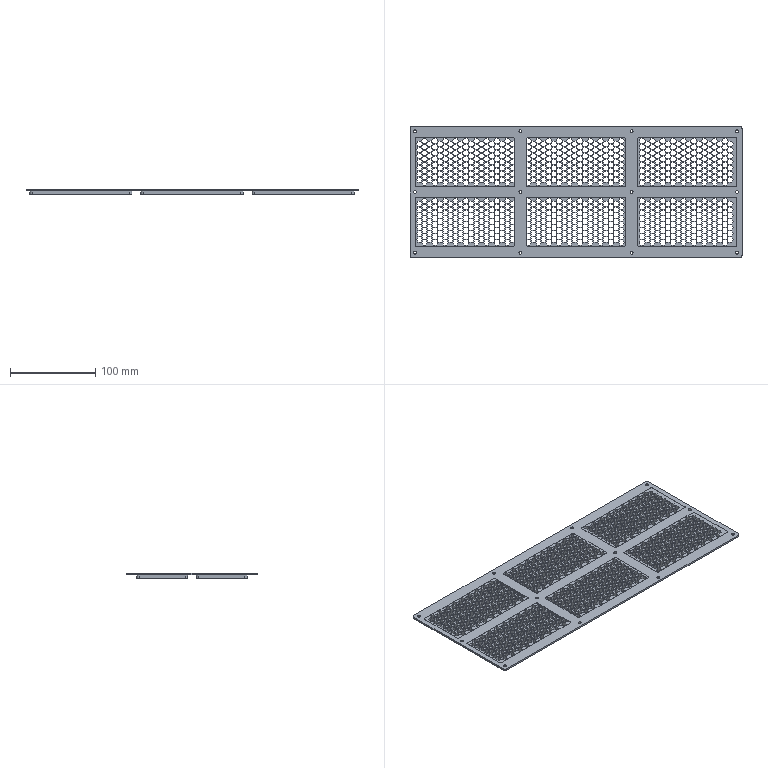NC program | NX | posted with a generic post
Lines 933 to 2108 of 7861:
(DRILLING_COPY_1 , TOOL : D4_CHAMFER)
N1822 T04 M6
N1824 G54
N1826 G17 G0 G90 X-183.338 Y56.437 S3000 M3
N1828 G43 Z30. H4
N1830 G94 G81 G98 Z-1.85 F200. R2.9
N1832 G80
N1834 G0 X-183.338 Y56.437 Z30.
(DRILLING_COPY_1_COPY_1 , TOOL : D4_CHAMFER)
N1836 X-171.218
N1838 G81 Z-1.85 F200. R2.9
N1840 G80
N1842 G0 X-171.218 Y56.437 Z30.
(DRILLING_COPY_1_COPY_2 , TOOL : D4_CHAMFER)
N1844 X-159.098
N1846 G81 Z-1.85 F200. R2.9
N1848 G80
N1850 G0 X-159.098 Y56.437 Z30.
(DRILLING_COPY_1_COPY_3 , TOOL : D4_CHAMFER)
N1852 X-146.978
N1854 G81 Z-1.85 F200. R2.9
N1856 G80
N1858 G0 X-146.978 Y56.437 Z30.
(DRILLING_COPY_1_COPY_4 , TOOL : D4_CHAMFER)
N1860 X-134.858
N1862 G81 Z-1.85 F200. R2.9
N1864 G80
N1866 G0 X-134.858 Y56.437 Z30.
(DRILLING_COPY_1_COPY_5 , TOOL : D4_CHAMFER)
N1868 X-122.738
N1870 G81 Z-1.85 F200. R2.9
N1872 G80
N1874 G0 X-122.738 Y56.437 Z30.
(DRILLING_COPY_1_COPY_6 , TOOL : D4_CHAMFER)
N1876 X-110.618
N1878 G81 Z-1.85 F200. R2.9
N1880 G80
N1882 G0 X-110.618 Y56.437 Z30.
(DRILLING_COPY_1_COPY_7 , TOOL : D4_CHAMFER)
N1884 X-98.498
N1886 G81 Z-1.85 F200. R2.9
N1888 G80
N1890 G0 X-98.498 Y56.437 Z30.
(DRILLING_COPY_1_COPY_8 , TOOL : D4_CHAMFER)
N1892 X-86.378
N1894 G81 Z-1.85 F200. R2.9
N1896 G80
N1898 G0 X-86.378 Y56.437 Z30.
(DRILLING_COPY_1_COPY_9 , TOOL : D4_CHAMFER)
N1900 X-183.338 Y49.437
N1902 G81 Z-1.85 F200. R2.9
N1904 G80
N1906 G0 X-183.338 Y49.437 Z30.
(DRILLING_COPY_1_COPY_1_COPY , TOOL : D4_CHAMFER)
N1908 X-171.218
N1910 G81 Z-1.85 F200. R2.9
N1912 G80
N1914 G0 X-171.218 Y49.437 Z30.
(DRILLING_COPY_1_COPY_2_COPY , TOOL : D4_CHAMFER)
N1916 X-159.098
N1918 G81 Z-1.85 F200. R2.9
N1920 G80
N1922 G0 X-159.098 Y49.437 Z30.
(DRILLING_COPY_1_COPY_3_COPY , TOOL : D4_CHAMFER)
N1924 X-146.978
N1926 G81 Z-1.85 F200. R2.9
N1928 G80
N1930 G0 X-146.978 Y49.437 Z30.
(DRILLING_COPY_1_COPY_4_COPY , TOOL : D4_CHAMFER)
N1932 X-134.858
N1934 G81 Z-1.85 F200. R2.9
N1936 G80
N1938 G0 X-134.858 Y49.437 Z30.
(DRILLING_COPY_1_COPY_5_COPY , TOOL : D4_CHAMFER)
N1940 X-122.738
N1942 G81 Z-1.85 F200. R2.9
N1944 G80
N1946 G0 X-122.738 Y49.437 Z30.
(DRILLING_COPY_1_COPY_6_COPY , TOOL : D4_CHAMFER)
N1948 X-110.618
N1950 G81 Z-1.85 F200. R2.9
N1952 G80
N1954 G0 X-110.618 Y49.437 Z30.
(DRILLING_COPY_1_COPY_7_COPY , TOOL : D4_CHAMFER)
N1956 X-98.498
N1958 G81 Z-1.85 F200. R2.9
N1960 G80
N1962 G0 X-98.498 Y49.437 Z30.
(DRILLING_COPY_1_COPY_8_COPY , TOOL : D4_CHAMFER)
N1964 X-86.378
N1966 G81 Z-1.85 F200. R2.9
N1968 G80
N1970 G0 X-86.378 Y49.437 Z30.
(DRILLING_COPY_1_COPY_10 , TOOL : D4_CHAMFER)
N1972 X-183.338 Y42.437
N1974 G81 Z-1.85 F200. R2.9
N1976 G80
N1978 G0 X-183.338 Y42.437 Z30.
(DRILLING_COPY_1_COPY_1_COPY_1 , TOOL : D4_CHAMFER)
N1980 X-171.218
N1982 G81 Z-1.85 F200. R2.9
N1984 G80
N1986 G0 X-171.218 Y42.437 Z30.
(DRILLING_COPY_1_COPY_2_COPY_1 , TOOL : D4_CHAMFER)
N1988 X-159.098
N1990 G81 Z-1.85 F200. R2.9
N1992 G80
N1994 G0 X-159.098 Y42.437 Z30.
(DRILLING_COPY_1_COPY_3_COPY_1 , TOOL : D4_CHAMFER)
N1996 X-146.978
N1998 G81 Z-1.85 F200. R2.9
N2000 G80
N2002 G0 X-146.978 Y42.437 Z30.
(DRILLING_COPY_1_COPY_4_COPY_1 , TOOL : D4_CHAMFER)
N2004 X-134.858
N2006 G81 Z-1.85 F200. R2.9
N2008 G80
N2010 G0 X-134.858 Y42.437 Z30.
(DRILLING_COPY_1_COPY_5_COPY_1 , TOOL : D4_CHAMFER)
N2012 X-122.738
N2014 G81 Z-1.85 F200. R2.9
N2016 G80
N2018 G0 X-122.738 Y42.437 Z30.
(DRILLING_COPY_1_COPY_6_COPY_1 , TOOL : D4_CHAMFER)
N2020 X-110.618
N2022 G81 Z-1.85 F200. R2.9
N2024 G80
N2026 G0 X-110.618 Y42.437 Z30.
(DRILLING_COPY_1_COPY_7_COPY_1 , TOOL : D4_CHAMFER)
N2028 X-98.498
N2030 G81 Z-1.85 F200. R2.9
N2032 G80
N2034 G0 X-98.498 Y42.437 Z30.
(DRILLING_COPY_1_COPY_8_COPY_1 , TOOL : D4_CHAMFER)
N2036 X-86.378
N2038 G81 Z-1.85 F200. R2.9
N2040 G80
N2042 G0 X-86.378 Y42.437 Z30.
(DRILLING_COPY_1_COPY_11 , TOOL : D4_CHAMFER)
N2044 X-183.338 Y35.437
N2046 G81 Z-1.85 F200. R2.9
N2048 G80
N2050 G0 X-183.338 Y35.437 Z30.
(DRILLING_COPY_1_COPY_1_COPY_2 , TOOL : D4_CHAMFER)
N2052 X-171.218
N2054 G81 Z-1.85 F200. R2.9
N2056 G80
N2058 G0 X-171.218 Y35.437 Z30.
(DRILLING_COPY_1_COPY_2_COPY_2 , TOOL : D4_CHAMFER)
N2060 X-159.098
N2062 G81 Z-1.85 F200. R2.9
N2064 G80
N2066 G0 X-159.098 Y35.437 Z30.
(DRILLING_COPY_1_COPY_3_COPY_2 , TOOL : D4_CHAMFER)
N2068 X-146.978
N2070 G81 Z-1.85 F200. R2.9
N2072 G80
N2074 G0 X-146.978 Y35.437 Z30.
(DRILLING_COPY_1_COPY_4_COPY_2 , TOOL : D4_CHAMFER)
N2076 X-134.858
N2078 G81 Z-1.85 F200. R2.9
N2080 G80
N2082 G0 X-134.858 Y35.437 Z30.
(DRILLING_COPY_1_COPY_5_COPY_2 , TOOL : D4_CHAMFER)
N2084 X-122.738
N2086 G81 Z-1.85 F200. R2.9
N2088 G80
N2090 G0 X-122.738 Y35.437 Z30.
(DRILLING_COPY_1_COPY_6_COPY_2 , TOOL : D4_CHAMFER)
N2092 X-110.618
N2094 G81 Z-1.85 F200. R2.9
N2096 G80
N2098 G0 X-110.618 Y35.437 Z30.
(DRILLING_COPY_1_COPY_7_COPY_2 , TOOL : D4_CHAMFER)
N2100 X-98.498
N2102 G81 Z-1.85 F200. R2.9
N2104 G80
N2106 G0 X-98.498 Y35.437 Z30.
(DRILLING_COPY_1_COPY_8_COPY_2 , TOOL : D4_CHAMFER)
N2108 X-86.378
N2110 G81 Z-1.85 F200. R2.9
N2112 G80
N2114 G0 X-86.378 Y35.437 Z30.
(DRILLING_COPY_1_COPY_12 , TOOL : D4_CHAMFER)
N2116 X-183.338 Y28.437
N2118 G81 Z-1.85 F200. R2.9
N2120 G80
N2122 G0 X-183.338 Y28.437 Z30.
(DRILLING_COPY_1_COPY_1_COPY_3 , TOOL : D4_CHAMFER)
N2124 X-171.218
N2126 G81 Z-1.85 F200. R2.9
N2128 G80
N2130 G0 X-171.218 Y28.437 Z30.
(DRILLING_COPY_1_COPY_2_COPY_3 , TOOL : D4_CHAMFER)
N2132 X-159.098
N2134 G81 Z-1.85 F200. R2.9
N2136 G80
N2138 G0 X-159.098 Y28.437 Z30.
(DRILLING_COPY_1_COPY_3_COPY_3 , TOOL : D4_CHAMFER)
N2140 X-146.978
N2142 G81 Z-1.85 F200. R2.9
N2144 G80
N2146 G0 X-146.978 Y28.437 Z30.
(DRILLING_COPY_1_COPY_4_COPY_3 , TOOL : D4_CHAMFER)
N2148 X-134.858
N2150 G81 Z-1.85 F200. R2.9
N2152 G80
N2154 G0 X-134.858 Y28.437 Z30.
(DRILLING_COPY_1_COPY_5_COPY_3 , TOOL : D4_CHAMFER)
N2156 X-122.738
N2158 G81 Z-1.85 F200. R2.9
N2160 G80
N2162 G0 X-122.738 Y28.437 Z30.
(DRILLING_COPY_1_COPY_6_COPY_3 , TOOL : D4_CHAMFER)
N2164 X-110.618
N2166 G81 Z-1.85 F200. R2.9
N2168 G80
N2170 G0 X-110.618 Y28.437 Z30.
(DRILLING_COPY_1_COPY_7_COPY_3 , TOOL : D4_CHAMFER)
N2172 X-98.498
N2174 G81 Z-1.85 F200. R2.9
N2176 G80
N2178 G0 X-98.498 Y28.437 Z30.
(DRILLING_COPY_1_COPY_8_COPY_3 , TOOL : D4_CHAMFER)
N2180 X-86.378
N2182 G81 Z-1.85 F200. R2.9
N2184 G80
N2186 G0 X-86.378 Y28.437 Z30.
(DRILLING_COPY_1_COPY_13 , TOOL : D4_CHAMFER)
N2188 X-183.338 Y21.437
N2190 G81 Z-1.85 F200. R2.9
N2192 G80
N2194 G0 X-183.338 Y21.437 Z30.
(DRILLING_COPY_1_COPY_1_COPY_4 , TOOL : D4_CHAMFER)
N2196 X-171.218
N2198 G81 Z-1.85 F200. R2.9
N2200 G80
N2202 G0 X-171.218 Y21.437 Z30.
(DRILLING_COPY_1_COPY_2_COPY_4 , TOOL : D4_CHAMFER)
N2204 X-159.098
N2206 G81 Z-1.85 F200. R2.9
N2208 G80
N2210 G0 X-159.098 Y21.437 Z30.
(DRILLING_COPY_1_COPY_3_COPY_4 , TOOL : D4_CHAMFER)
N2212 X-146.978
N2214 G81 Z-1.85 F200. R2.9
N2216 G80
N2218 G0 X-146.978 Y21.437 Z30.
(DRILLING_COPY_1_COPY_4_COPY_4 , TOOL : D4_CHAMFER)
N2220 X-134.858
N2222 G81 Z-1.85 F200. R2.9
N2224 G80
N2226 G0 X-134.858 Y21.437 Z30.
(DRILLING_COPY_1_COPY_5_COPY_4 , TOOL : D4_CHAMFER)
N2228 X-122.738
N2230 G81 Z-1.85 F200. R2.9
N2232 G80
N2234 G0 X-122.738 Y21.437 Z30.
(DRILLING_COPY_1_COPY_6_COPY_4 , TOOL : D4_CHAMFER)
N2236 X-110.618
N2238 G81 Z-1.85 F200. R2.9
N2240 G80
N2242 G0 X-110.618 Y21.437 Z30.
(DRILLING_COPY_1_COPY_7_COPY_4 , TOOL : D4_CHAMFER)
N2244 X-98.498
N2246 G81 Z-1.85 F200. R2.9
N2248 G80
N2250 G0 X-98.498 Y21.437 Z30.
(DRILLING_COPY_1_COPY_8_COPY_4 , TOOL : D4_CHAMFER)
N2252 X-86.378
N2254 G81 Z-1.85 F200. R2.9
N2256 G80
N2258 G0 X-86.378 Y21.437 Z30.
(DRILLING_COPY_1_COPY_14 , TOOL : D4_CHAMFER)
N2260 X-183.338 Y14.437
N2262 G81 Z-1.85 F200. R2.9
N2264 G80
N2266 G0 X-183.338 Y14.437 Z30.
(DRILLING_COPY_1_COPY_1_COPY_5 , TOOL : D4_CHAMFER)
N2268 X-171.218
N2270 G81 Z-1.85 F200. R2.9
N2272 G80
N2274 G0 X-171.218 Y14.437 Z30.
(DRILLING_COPY_1_COPY_2_COPY_5 , TOOL : D4_CHAMFER)
N2276 X-159.098
N2278 G81 Z-1.85 F200. R2.9
N2280 G80
N2282 G0 X-159.098 Y14.437 Z30.
(DRILLING_COPY_1_COPY_3_COPY_5 , TOOL : D4_CHAMFER)
N2284 X-146.978
N2286 G81 Z-1.85 F200. R2.9
N2288 G80
N2290 G0 X-146.978 Y14.437 Z30.
(DRILLING_COPY_1_COPY_4_COPY_5 , TOOL : D4_CHAMFER)
N2292 X-134.858
N2294 G81 Z-1.85 F200. R2.9
N2296 G80
N2298 G0 X-134.858 Y14.437 Z30.
(DRILLING_COPY_1_COPY_5_COPY_5 , TOOL : D4_CHAMFER)
N2300 X-122.738
N2302 G81 Z-1.85 F200. R2.9
N2304 G80
N2306 G0 X-122.738 Y14.437 Z30.
(DRILLING_COPY_1_COPY_6_COPY_5 , TOOL : D4_CHAMFER)
N2308 X-110.618
N2310 G81 Z-1.85 F200. R2.9
N2312 G80
N2314 G0 X-110.618 Y14.437 Z30.
(DRILLING_COPY_1_COPY_7_COPY_5 , TOOL : D4_CHAMFER)
N2316 X-98.498
N2318 G81 Z-1.85 F200. R2.9
N2320 G80
N2322 G0 X-98.498 Y14.437 Z30.
(DRILLING_COPY_1_COPY_8_COPY_5 , TOOL : D4_CHAMFER)
N2324 X-86.378
N2326 G81 Z-1.85 F200. R2.9
N2328 G80
N2330 G0 X-86.378 Y14.437 Z30.
(DRILLING_COPY_1_COPY , TOOL : D4_CHAMFER)
N2332 X-177.276 Y59.937
N2334 G81 Z-1.85 F200. R2.9
N2336 G80
N2338 G0 X-177.276 Y59.937 Z30.
(DRILLING_COPY_1_COPY_COPY , TOOL : D4_CHAMFER)
N2340 X-165.156
N2342 G81 Z-1.85 F200. R2.9
N2344 G80
N2346 G0 X-165.156 Y59.937 Z30.
(DRILLING_COPY_1_COPY_COPY_1 , TOOL : D4_CHAMFER)
N2348 X-153.036
N2350 G81 Z-1.85 F200. R2.9
N2352 G80
N2354 G0 X-153.036 Y59.937 Z30.
(DRILLING_COPY_1_COPY_COPY_2 , TOOL : D4_CHAMFER)
N2356 X-140.916
N2358 G81 Z-1.85 F200. R2.9
N2360 G80
N2362 G0 X-140.916 Y59.937 Z30.
(DRILLING_COPY_1_COPY_COPY_3 , TOOL : D4_CHAMFER)
N2364 X-128.796
N2366 G81 Z-1.85 F200. R2.9
N2368 G80
N2370 G0 X-128.796 Y59.937 Z30.
(DRILLING_COPY_1_COPY_COPY_4 , TOOL : D4_CHAMFER)
N2372 X-116.676
N2374 G81 Z-1.85 F200. R2.9
N2376 G80
N2378 G0 X-116.676 Y59.937 Z30.
(DRILLING_COPY_1_COPY_COPY_5 , TOOL : D4_CHAMFER)
N2380 X-104.556
N2382 G81 Z-1.85 F200. R2.9
N2384 G80
N2386 G0 X-104.556 Y59.937 Z30.
(DRILLING_COPY_1_COPY_COPY_6 , TOOL : D4_CHAMFER)
N2388 X-92.436
N2390 G81 Z-1.85 F200. R2.9
N2392 G80
N2394 G0 X-92.436 Y59.937 Z30.
(DRILLING_COPY_1_COPY_COPY_7 , TOOL : D4_CHAMFER)
N2396 X-80.316
N2398 G81 Z-1.85 F200. R2.9
N2400 G80
N2402 G0 X-80.316 Y59.937 Z30.
(DRILLING_COPY_1_COPY_COPY_8 , TOOL : D4_CHAMFER)
N2404 X-177.276 Y52.937
N2406 G81 Z-1.85 F200. R2.9
N2408 G80
N2410 G0 X-177.276 Y52.937 Z30.
(DRILLING_COPY_1_COPY_COPY_COPY , TOOL : D4_CHAMFER)
N2412 X-165.156
N2414 G81 Z-1.85 F200. R2.9
N2416 G80
N2418 G0 X-165.156 Y52.937 Z30.
(DRILLING_COPY_1_COPY_COPY_1_COPY , TOOL : D4_CHAMFER)
N2420 X-153.036
N2422 G81 Z-1.85 F200. R2.9
N2424 G80
N2426 G0 X-153.036 Y52.937 Z30.
(DRILLING_COPY_1_COPY_COPY_2_COPY , TOOL : D4_CHAMFER)
N2428 X-140.916
N2430 G81 Z-1.85 F200. R2.9
N2432 G80
N2434 G0 X-140.916 Y52.937 Z30.
(DRILLING_COPY_1_COPY_COPY_3_COPY , TOOL : D4_CHAMFER)
N2436 X-128.796
N2438 G81 Z-1.85 F200. R2.9
N2440 G80
N2442 G0 X-128.796 Y52.937 Z30.
(DRILLING_COPY_1_COPY_COPY_4_COPY , TOOL : D4_CHAMFER)
N2444 X-116.676
N2446 G81 Z-1.85 F200. R2.9
N2448 G80
N2450 G0 X-116.676 Y52.937 Z30.
(DRILLING_COPY_1_COPY_COPY_5_COPY , TOOL : D4_CHAMFER)
N2452 X-104.556
N2454 G81 Z-1.85 F200. R2.9
N2456 G80
N2458 G0 X-104.556 Y52.937 Z30.
(DRILLING_COPY_1_COPY_COPY_6_COPY , TOOL : D4_CHAMFER)
N2460 X-92.436
N2462 G81 Z-1.85 F200. R2.9
N2464 G80
N2466 G0 X-92.436 Y52.937 Z30.
(DRILLING_COPY_1_COPY_COPY_7_COPY , TOOL : D4_CHAMFER)
N2468 X-80.316
N2470 G81 Z-1.85 F200. R2.9
N2472 G80
N2474 G0 X-80.316 Y52.937 Z30.
(DRILLING_COPY_1_COPY_COPY_9 , TOOL : D4_CHAMFER)
N2476 X-177.276 Y45.937
N2478 G81 Z-1.85 F200. R2.9
N2480 G80
N2482 G0 X-177.276 Y45.937 Z30.
(DRILLING_COPY_1_COPY_COPY_COPY_1 , TOOL : D4_CHAMFER)
N2484 X-165.156
N2486 G81 Z-1.85 F200. R2.9
N2488 G80
N2490 G0 X-165.156 Y45.937 Z30.
(DRILLING_COPY_1_COPY_COPY_1_COPY_1 , TOOL : D4_CHAMFER)
N2492 X-153.036
N2494 G81 Z-1.85 F200. R2.9
N2496 G80
N2498 G0 X-153.036 Y45.937 Z30.
(DRILLING_COPY_1_COPY_COPY_2_COPY_1 , TOOL : D4_CHAMFER)
N2500 X-140.916
N2502 G81 Z-1.85 F200. R2.9
N2504 G80
N2506 G0 X-140.916 Y45.937 Z30.
(DRILLING_COPY_1_COPY_COPY_3_COPY_1 , TOOL : D4_CHAMFER)
N2508 X-128.796
N2510 G81 Z-1.85 F200. R2.9
N2512 G80
N2514 G0 X-128.796 Y45.937 Z30.
(DRILLING_COPY_1_COPY_COPY_4_COPY_1 , TOOL : D4_CHAMFER)
N2516 X-116.676
N2518 G81 Z-1.85 F200. R2.9
N2520 G80
N2522 G0 X-116.676 Y45.937 Z30.
(DRILLING_COPY_1_COPY_COPY_5_COPY_1 , TOOL : D4_CHAMFER)
N2524 X-104.556
N2526 G81 Z-1.85 F200. R2.9
N2528 G80
N2530 G0 X-104.556 Y45.937 Z30.
(DRILLING_COPY_1_COPY_COPY_6_COPY_1 , TOOL : D4_CHAMFER)
N2532 X-92.436
N2534 G81 Z-1.85 F200. R2.9
N2536 G80
N2538 G0 X-92.436 Y45.937 Z30.
(DRILLING_COPY_1_COPY_COPY_7_COPY_1 , TOOL : D4_CHAMFER)
N2540 X-80.316
N2542 G81 Z-1.85 F200. R2.9
N2544 G80
N2546 G0 X-80.316 Y45.937 Z30.
(DRILLING_COPY_1_COPY_COPY_10 , TOOL : D4_CHAMFER)
N2548 X-177.276 Y38.937
N2550 G81 Z-1.85 F200. R2.9
N2552 G80
N2554 G0 X-177.276 Y38.937 Z30.
(DRILLING_COPY_1_COPY_COPY_COPY_2 , TOOL : D4_CHAMFER)
N2556 X-165.156
N2558 G81 Z-1.85 F200. R2.9
N2560 G80
N2562 G0 X-165.156 Y38.937 Z30.
(DRILLING_COPY_1_COPY_COPY_1_COPY_2 , TOOL : D4_CHAMFER)
N2564 X-153.036
N2566 G81 Z-1.85 F200. R2.9
N2568 G80
N2570 G0 X-153.036 Y38.937 Z30.
(DRILLING_COPY_1_COPY_COPY_2_COPY_2 , TOOL : D4_CHAMFER)
N2572 X-140.916
N2574 G81 Z-1.85 F200. R2.9
N2576 G80
N2578 G0 X-140.916 Y38.937 Z30.
(DRILLING_COPY_1_COPY_COPY_3_COPY_2 , TOOL : D4_CHAMFER)
N2580 X-128.796
N2582 G81 Z-1.85 F200. R2.9
N2584 G80
N2586 G0 X-128.796 Y38.937 Z30.
(DRILLING_COPY_1_COPY_COPY_4_COPY_2 , TOOL : D4_CHAMFER)
N2588 X-116.676
N2590 G81 Z-1.85 F200. R2.9
N2592 G80
N2594 G0 X-116.676 Y38.937 Z30.
(DRILLING_COPY_1_COPY_COPY_5_COPY_2 , TOOL : D4_CHAMFER)
N2596 X-104.556
N2598 G81 Z-1.85 F200. R2.9
N2600 G80
N2602 G0 X-104.556 Y38.937 Z30.
(DRILLING_COPY_1_COPY_COPY_6_COPY_2 , TOOL : D4_CHAMFER)
N2604 X-92.436
N2606 G81 Z-1.85 F200. R2.9
N2608 G80
N2610 G0 X-92.436 Y38.937 Z30.
(DRILLING_COPY_1_COPY_COPY_7_COPY_2 , TOOL : D4_CHAMFER)
N2612 X-80.316
N2614 G81 Z-1.85 F200. R2.9
N2616 G80
N2618 G0 X-80.316 Y38.937 Z30.
(DRILLING_COPY_1_COPY_COPY_11 , TOOL : D4_CHAMFER)
N2620 X-177.276 Y31.937
N2622 G81 Z-1.85 F200. R2.9
N2624 G80
N2626 G0 X-177.276 Y31.937 Z30.
(DRILLING_COPY_1_COPY_COPY_COPY_3 , TOOL : D4_CHAMFER)
N2628 X-165.156
N2630 G81 Z-1.85 F200. R2.9
N2632 G80
N2634 G0 X-165.156 Y31.937 Z30.
(DRILLING_COPY_1_COPY_COPY_1_COPY_3 , TOOL : D4_CHAMFER)
N2636 X-153.036
N2638 G81 Z-1.85 F200. R2.9
N2640 G80
N2642 G0 X-153.036 Y31.937 Z30.
(DRILLING_COPY_1_COPY_COPY_2_COPY_3 , TOOL : D4_CHAMFER)
N2644 X-140.916
N2646 G81 Z-1.85 F200. R2.9
N2648 G80
N2650 G0 X-140.916 Y31.937 Z30.
(DRILLING_COPY_1_COPY_COPY_3_COPY_3 , TOOL : D4_CHAMFER)
N2652 X-128.796
N2654 G81 Z-1.85 F200. R2.9
N2656 G80
N2658 G0 X-128.796 Y31.937 Z30.
(DRILLING_COPY_1_COPY_COPY_4_COPY_3 , TOOL : D4_CHAMFER)
N2660 X-116.676
N2662 G81 Z-1.85 F200. R2.9
N2664 G80
N2666 G0 X-116.676 Y31.937 Z30.
(DRILLING_COPY_1_COPY_COPY_5_COPY_3 , TOOL : D4_CHAMFER)
N2668 X-104.556
N2670 G81 Z-1.85 F200. R2.9
N2672 G80
N2674 G0 X-104.556 Y31.937 Z30.
(DRILLING_COPY_1_COPY_COPY_6_COPY_3 , TOOL : D4_CHAMFER)
N2676 X-92.436
N2678 G81 Z-1.85 F200. R2.9
N2680 G80
N2682 G0 X-92.436 Y31.937 Z30.
(DRILLING_COPY_1_COPY_COPY_7_COPY_3 , TOOL : D4_CHAMFER)
N2684 X-80.316
N2686 G81 Z-1.85 F200. R2.9
N2688 G80
N2690 G0 X-80.316 Y31.937 Z30.
(DRILLING_COPY_1_COPY_COPY_12 , TOOL : D4_CHAMFER)
N2692 X-177.276 Y24.937
N2694 G81 Z-1.85 F200. R2.9
N2696 G80
N2698 G0 X-177.276 Y24.937 Z30.
(DRILLING_COPY_1_COPY_COPY_COPY_4 , TOOL : D4_CHAMFER)
N2700 X-165.156
N2702 G81 Z-1.85 F200. R2.9
N2704 G80
N2706 G0 X-165.156 Y24.937 Z30.
(DRILLING_COPY_1_COPY_COPY_1_COPY_4 , TOOL : D4_CHAMFER)
N2708 X-153.036
N2710 G81 Z-1.85 F200. R2.9
N2712 G80
N2714 G0 X-153.036 Y24.937 Z30.
(DRILLING_COPY_1_COPY_COPY_2_COPY_4 , TOOL : D4_CHAMFER)
N2716 X-140.916
N2718 G81 Z-1.85 F200. R2.9
N2720 G80
N2722 G0 X-140.916 Y24.937 Z30.
(DRILLING_COPY_1_COPY_COPY_3_COPY_4 , TOOL : D4_CHAMFER)
N2724 X-128.796
N2726 G81 Z-1.85 F200. R2.9
N2728 G80
N2730 G0 X-128.796 Y24.937 Z30.
(DRILLING_COPY_1_COPY_COPY_4_COPY_4 , TOOL : D4_CHAMFER)
N2732 X-116.676
N2734 G81 Z-1.85 F200. R2.9
N2736 G80
N2738 G0 X-116.676 Y24.937 Z30.
(DRILLING_COPY_1_COPY_COPY_5_COPY_4 , TOOL : D4_CHAMFER)
N2740 X-104.556
N2742 G81 Z-1.85 F200. R2.9
N2744 G80
N2746 G0 X-104.556 Y24.937 Z30.
(DRILLING_COPY_1_COPY_COPY_6_COPY_4 , TOOL : D4_CHAMFER)
N2748 X-92.436
N2750 G81 Z-1.85 F200. R2.9
N2752 G80
N2754 G0 X-92.436 Y24.937 Z30.
(DRILLING_COPY_1_COPY_COPY_7_COPY_4 , TOOL : D4_CHAMFER)
N2756 X-80.316
N2758 G81 Z-1.85 F200. R2.9
N2760 G80
N2762 G0 X-80.316 Y24.937 Z30.
(DRILLING_COPY_1_COPY_COPY_13 , TOOL : D4_CHAMFER)
N2764 X-177.276 Y17.937
N2766 G81 Z-1.85 F200. R2.9
N2768 G80
N2770 G0 X-177.276 Y17.937 Z30.
(DRILLING_COPY_1_COPY_COPY_COPY_5 , TOOL : D4_CHAMFER)
N2772 X-165.156
N2774 G81 Z-1.85 F200. R2.9
N2776 G80
N2778 G0 X-165.156 Y17.937 Z30.
(DRILLING_COPY_1_COPY_COPY_1_COPY_5 , TOOL : D4_CHAMFER)
N2780 X-153.036
N2782 G81 Z-1.85 F200. R2.9
N2784 G80
N2786 G0 X-153.036 Y17.937 Z30.
(DRILLING_COPY_1_COPY_COPY_2_COPY_5 , TOOL : D4_CHAMFER)
N2788 X-140.916
N2790 G81 Z-1.85 F200. R2.9
N2792 G80
N2794 G0 X-140.916 Y17.937 Z30.
(DRILLING_COPY_1_COPY_COPY_3_COPY_5 , TOOL : D4_CHAMFER)
N2796 X-128.796
N2798 G81 Z-1.85 F200. R2.9
N2800 G80
N2802 G0 X-128.796 Y17.937 Z30.
(DRILLING_COPY_1_COPY_COPY_4_COPY_5 , TOOL : D4_CHAMFER)
N2804 X-116.676
N2806 G81 Z-1.85 F200. R2.9
N2808 G80
N2810 G0 X-116.676 Y17.937 Z30.
(DRILLING_COPY_1_COPY_COPY_5_COPY_5 , TOOL : D4_CHAMFER)
N2812 X-104.556
N2814 G81 Z-1.85 F200. R2.9
N2816 G80
N2818 G0 X-104.556 Y17.937 Z30.
(DRILLING_COPY_1_COPY_COPY_6_COPY_5 , TOOL : D4_CHAMFER)
N2820 X-92.436
N2822 G81 Z-1.85 F200. R2.9
N2824 G80
N2826 G0 X-92.436 Y17.937 Z30.
(DRILLING_COPY_1_COPY_COPY_7_COPY_5 , TOOL : D4_CHAMFER)
N2828 X-80.316
N2830 G81 Z-1.85 F200. R2.9
N2832 G80
N2834 G0 X-80.316 Y17.937 Z30.
(DRILLING_COPY_1_COPY_COPY_14 , TOOL : D4_CHAMFER)
N2836 X-177.276 Y10.937
N2838 G81 Z-1.85 F200. R2.9
N2840 G80
N2842 G0 X-177.276 Y10.937 Z30.
(DRILLING_COPY_1_COPY_COPY_COPY_6 , TOOL : D4_CHAMFER)
N2844 X-165.156
N2846 G81 Z-1.85 F200. R2.9
N2848 G80
N2850 G0 X-165.156 Y10.937 Z30.
(DRILLING_COPY_1_COPY_COPY_1_COPY_6 , TOOL : D4_CHAMFER)
N2852 X-153.036
N2854 G81 Z-1.85 F200. R2.9
N2856 G80
N2858 G0 X-153.036 Y10.937 Z30.
(DRILLING_COPY_1_COPY_COPY_2_COPY_6 , TOOL : D4_CHAMFER)
N2860 X-140.916
N2862 G81 Z-1.85 F200. R2.9
N2864 G80
N2866 G0 X-140.916 Y10.937 Z30.
(DRILLING_COPY_1_COPY_COPY_3_COPY_6 , TOOL : D4_CHAMFER)
N2868 X-128.796
N2870 G81 Z-1.85 F200. R2.9
N2872 G80
N2874 G0 X-128.796 Y10.937 Z30.
(DRILLING_COPY_1_COPY_COPY_4_COPY_6 , TOOL : D4_CHAMFER)
N2876 X-116.676
N2878 G81 Z-1.85 F200. R2.9
N2880 G80
N2882 G0 X-116.676 Y10.937 Z30.
(DRILLING_COPY_1_COPY_COPY_5_COPY_6 , TOOL : D4_CHAMFER)
N2884 X-104.556
N2886 G81 Z-1.85 F200. R2.9
N2888 G80
N2890 G0 X-104.556 Y10.937 Z30.
(DRILLING_COPY_1_COPY_COPY_6_COPY_6 , TOOL : D4_CHAMFER)
N2892 X-92.436
N2894 G81 Z-1.85 F200. R2.9
N2896 G80
N2898 G0 X-92.436 Y10.937 Z30.
(DRILLING_COPY_1_COPY_COPY_7_COPY_6 , TOOL : D4_CHAMFER)
N2900 X-80.316
N2902 G81 Z-1.85 F200. R2.9
N2904 G80
N2906 G0 X-80.316 Y10.937 Z30.
(DRILLING_COPY_1_COPY_15 , TOOL : D4_CHAMFER)
N2908 X-74.218 Y56.437
N2910 G81 Z-1.85 F200. R2.9
N2912 G80
N2914 G0 X-74.218 Y56.437 Z30.
(DRILLING_COPY_1_COPY_15_COPY , TOOL : D4_CHAMFER)
N2916 Y49.437
N2918 G81 Z-1.85 F200. R2.9
N2920 G80
N2922 G0 X-74.218 Y49.437 Z30.
(DRILLING_COPY_1_COPY_15_COPY_1 , TOOL : D4_CHAMFER)
N2924 Y42.437
N2926 G81 Z-1.85 F200. R2.9
N2928 G80
N2930 G0 X-74.218 Y42.437 Z30.
(DRILLING_COPY_1_COPY_15_COPY_2 , TOOL : D4_CHAMFER)
N2932 Y35.437
N2934 G81 Z-1.85 F200. R2.9
N2936 G80
N2938 G0 X-74.218 Y35.437 Z30.
(DRILLING_COPY_1_COPY_15_COPY_3 , TOOL : D4_CHAMFER)
N2940 Y28.437
N2942 G81 Z-1.85 F200. R2.9
N2944 G80
N2946 G0 X-74.218 Y28.437 Z30.
(DRILLING_COPY_1_COPY_15_COPY_4 , TOOL : D4_CHAMFER)
N2948 Y21.437
N2950 G81 Z-1.85 F200. R2.9
N2952 G80
N2954 G0 X-74.218 Y21.437 Z30.
(DRILLING_COPY_1_COPY_15_COPY_5 , TOOL : D4_CHAMFER)
N2956 Y14.437
N2958 G81 Z-1.85 F200. R2.9
N2960 G80
N2962 G0 X-74.218 Y14.437 Z30.
(DRILLING_COPY_1_COPY_15_COPY_6 , TOOL : D4_CHAMFER)
N2964 X-183.338 Y-55.563
N2966 G81 Z-1.85 F200. R2.9
N2968 G80
N2970 G0 X-183.338 Y-55.563 Z30.
(DRILLING_COPY_1_COPY_15_COPY_6_COPY , TOOL : D4_CHAMFER)
N2972 Y-48.563
N2974 G81 Z-1.85 F200. R2.9
N2976 G80
N2978 G0 X-183.338 Y-48.563 Z30.
(DRILLING_COPY_1_COPY_15_COPY_6_COPY_1 , TOOL : D4_CHAMFER)
N2980 Y-41.563
N2982 G81 Z-1.85 F200. R2.9
N2984 G80
N2986 G0 X-183.338 Y-41.563 Z30.
(DRILLING_COPY_1_COPY_15_COPY_6_COPY_2 , TOOL : D4_CHAMFER)
N2988 Y-34.563
N2990 G81 Z-1.85 F200. R2.9
N2992 G80
N2994 G0 X-183.338 Y-34.563 Z30.
(DRILLING_COPY_1_COPY_15_COPY_6_COPY_3 , TOOL : D4_CHAMFER)
N2996 Y-27.563
N2998 G81 Z-1.85 F200. R2.9
N3000 G80
N3002 G0 X-183.338 Y-27.563 Z30.
(DRILLING_COPY_1_COPY_15_COPY_6_COPY_4 , TOOL : D4_CHAMFER)
N3004 Y-20.563
N3006 G81 Z-1.85 F200. R2.9
N3008 G80
N3010 G0 X-183.338 Y-20.563 Z30.
(DRILLING_COPY_1_COPY_15_COPY_6_COPY_5 , TOOL : D4_CHAMFER)
N3012 Y-13.563
N3014 G81 Z-1.85 F200. R2.9
N3016 G80
N3018 G0 X-183.338 Y-13.563 Z30.
(DRILLING_COPY_1_COPY_15_COPY_6_COPY_6 , TOOL : D4_CHAMFER)
N3020 X-171.218 Y-55.563
N3022 G81 Z-1.85 F200. R2.9
N3024 G80
N3026 G0 X-171.218 Y-55.563 Z30.
(DRILLING_COPY_1_COPY_15_COPY_6_COPY_COPY , TOOL : D4_CHAMFER)
N3028 Y-48.563
N3030 G81 Z-1.85 F200. R2.9
N3032 G80
N3034 G0 X-171.218 Y-48.563 Z30.
(DRILLING_COPY_1_COPY_15_COPY_6_COPY_1_COPY , TOOL : D4_CHAMFER)
N3036 Y-41.563
N3038 G81 Z-1.85 F200. R2.9
N3040 G80
N3042 G0 X-171.218 Y-41.563 Z30.
(DRILLING_COPY_1_COPY_15_COPY_6_COPY_2_COPY , TOOL : D4_CHAMFER)
N3044 Y-34.563
N3046 G81 Z-1.85 F200. R2.9
N3048 G80
N3050 G0 X-171.218 Y-34.563 Z30.
(DRILLING_COPY_1_COPY_15_COPY_6_COPY_3_COPY , TOOL : D4_CHAMFER)
N3052 Y-27.563
N3054 G81 Z-1.85 F200. R2.9
N3056 G80
N3058 G0 X-171.218 Y-27.563 Z30.
(DRILLING_COPY_1_COPY_15_COPY_6_COPY_4_COPY , TOOL : D4_CHAMFER)
N3060 Y-20.563
N3062 G81 Z-1.85 F200. R2.9
N3064 G80
N3066 G0 X-171.218 Y-20.563 Z30.
(DRILLING_COPY_1_COPY_15_COPY_6_COPY_5_COPY , TOOL : D4_CHAMFER)
N3068 Y-13.563
N3070 G81 Z-1.85 F200. R2.9
N3072 G80
N3074 G0 X-171.218 Y-13.563 Z30.
(DRILLING_COPY_1_COPY_15_COPY_6_COPY_7 , TOOL : D4_CHAMFER)
N3076 X-159.098 Y-55.563
N3078 G81 Z-1.85 F200. R2.9
N3080 G80
N3082 G0 X-159.098 Y-55.563 Z30.
(DRILLING_COPY_1_COPY_15_COPY_6_COPY_COPY_1 , TOOL : D4_CHAMFER)
N3084 Y-48.563
N3086 G81 Z-1.85 F200. R2.9
N3088 G80
N3090 G0 X-159.098 Y-48.563 Z30.
(DRILLING_COPY_1_COPY_15_COPY_6_COPY_1_COPY_1 , TOOL : D4_CHAMFER)
N3092 Y-41.563
N3094 G81 Z-1.85 F200. R2.9
N3096 G80
N3098 G0 X-159.098 Y-41.563 Z30.
(DRILLING_COPY_1_COPY_15_COPY_6_COPY_2_COPY_1 , TOOL : D4_CHAMFER)
N3100 Y-34.563
N3102 G81 Z-1.85 F200. R2.9
N3104 G80
N3106 G0 X-159.098 Y-34.563 Z30.
(DRILLING_COPY_1_COPY_15_COPY_6_COPY_3_COPY_1 , TOOL : D4_CHAMFER)
N3108 Y-27.563
N3110 G81 Z-1.85 F200. R2.9
N3112 G80
N3114 G0 X-159.098 Y-27.563 Z30.
(DRILLING_COPY_1_COPY_15_COPY_6_COPY_4_COPY_1 , TOOL : D4_CHAMFER)
N3116 Y-20.563
N3118 G81 Z-1.85 F200. R2.9
N3120 G80
N3122 G0 X-159.098 Y-20.563 Z30.
(DRILLING_COPY_1_COPY_15_COPY_6_COPY_5_COPY_1 , TOOL : D4_CHAMFER)
N3124 Y-13.563
N3126 G81 Z-1.85 F200. R2.9
N3128 G80
N3130 G0 X-159.098 Y-13.563 Z30.
(DRILLING_COPY_1_COPY_15_COPY_6_COPY_8 , TOOL : D4_CHAMFER)
N3132 X-146.978 Y-55.563
N3134 G81 Z-1.85 F200. R2.9
N3136 G80
N3138 G0 X-146.978 Y-55.563 Z30.
(DRILLING_COPY_1_COPY_15_COPY_6_COPY_COPY_2 , TOOL : D4_CHAMFER)
N3140 Y-48.563
N3142 G81 Z-1.85 F200. R2.9
N3144 G80
N3146 G0 X-146.978 Y-48.563 Z30.
(DRILLING_COPY_1_COPY_15_COPY_6_COPY_1_COPY_2 , TOOL : D4_CHAMFER)
N3148 Y-41.563
N3150 G81 Z-1.85 F200. R2.9
N3152 G80
N3154 G0 X-146.978 Y-41.563 Z30.
(DRILLING_COPY_1_COPY_15_COPY_6_COPY_2_COPY_2 , TOOL : D4_CHAMFER)
N3156 Y-34.563
N3158 G81 Z-1.85 F200. R2.9
N3160 G80
N3162 G0 X-146.978 Y-34.563 Z30.
(DRILLING_COPY_1_COPY_15_COPY_6_COPY_3_COPY_2 , TOOL : D4_CHAMFER)
N3164 Y-27.563